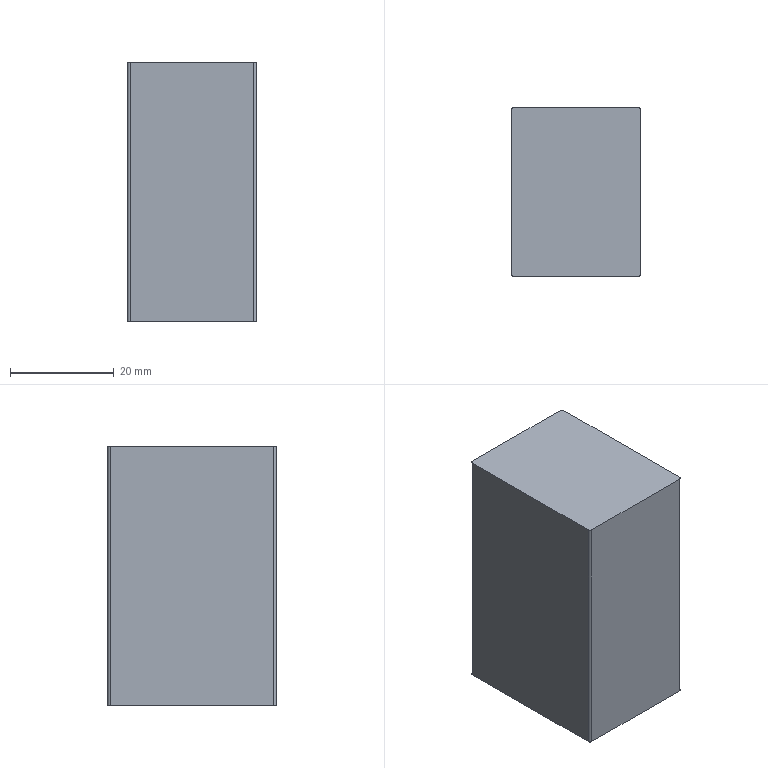Part | NX | features BREP 1 | 1 solid | 10 faces | box 24.892 x 32.505 x 50 mm | volume 40445 mm3 | plane 6 | cylinder 4 | commonest cylinder face diameters 1 x4
STEP:
#1=CARTESIAN_POINT('',(-11.946,16.253,-40.6));
#2=VERTEX_POINT('',#1);
#3=CARTESIAN_POINT('',(-12.446,15.753,-40.6));
#4=VERTEX_POINT('',#3);
#5=CARTESIAN_POINT('',(-11.946,15.753,-40.6));
#6=DIRECTION('',(0.,0.,1.));
#7=DIRECTION('',(1.,0.,0.));
#8=AXIS2_PLACEMENT_3D('',#5,#6,#7);
#9=CIRCLE('',#8,0.5);
#10=EDGE_CURVE('',#2,#4,#9,.T.);
#11=ORIENTED_EDGE('',*,*,#10,.F.);
#12=CARTESIAN_POINT('',(-11.946,16.253,-90.6));
#13=VERTEX_POINT('',#12);
#14=CARTESIAN_POINT('',(-11.946,16.253,-90.6));
#15=DIRECTION('',(0.,0.,1.));
#16=VECTOR('',#15,1000.);
#17=LINE('',#14,#16);
#18=EDGE_CURVE('',#13,#2,#17,.T.);
#19=ORIENTED_EDGE('',*,*,#18,.F.);
#20=CARTESIAN_POINT('',(-12.446,15.753,-90.6));
#21=VERTEX_POINT('',#20);
#22=CARTESIAN_POINT('',(-11.946,15.753,-90.6));
#23=DIRECTION('',(0.,0.,1.));
#24=DIRECTION('',(1.,0.,0.));
#25=AXIS2_PLACEMENT_3D('',#22,#23,#24);
#26=CIRCLE('',#25,0.5);
#27=EDGE_CURVE('',#13,#21,#26,.T.);
#28=ORIENTED_EDGE('',*,*,#27,.T.);
#29=CARTESIAN_POINT('',(-12.446,15.753,-90.6));
#30=DIRECTION('',(0.,0.,1.));
#31=VECTOR('',#30,1000.);
#32=LINE('',#29,#31);
#33=EDGE_CURVE('',#21,#4,#32,.T.);
#34=ORIENTED_EDGE('',*,*,#33,.T.);
#35=EDGE_LOOP('',(#11,#19,#28,#34));
#36=FACE_BOUND('',#35,.T.);
#37=CARTESIAN_POINT('',(-11.946,15.753,-90.6));
#38=DIRECTION('',(0.,0.,1.));
#39=DIRECTION('',(-1.,0.,0.));
#40=AXIS2_PLACEMENT_3D('',#37,#38,#39);
#41=CYLINDRICAL_SURFACE('',#40,0.5);
#42=ADVANCED_FACE('',(#36),#41,.T.);
#43=CARTESIAN_POINT('',(-12.446,-15.753,-40.6));
#44=VERTEX_POINT('',#43);
#45=CARTESIAN_POINT('',(-12.446,-15.753,-40.6));
#46=DIRECTION('',(0.,1.,0.));
#47=VECTOR('',#46,1000.);
#48=LINE('',#45,#47);
#49=EDGE_CURVE('',#44,#4,#48,.T.);
#50=ORIENTED_EDGE('',*,*,#49,.T.);
#51=ORIENTED_EDGE('',*,*,#33,.F.);
#52=CARTESIAN_POINT('',(-12.446,-15.753,-90.6));
#53=VERTEX_POINT('',#52);
#54=CARTESIAN_POINT('',(-12.446,-15.753,-90.6));
#55=DIRECTION('',(0.,1.,0.));
#56=VECTOR('',#55,1000.);
#57=LINE('',#54,#56);
#58=EDGE_CURVE('',#53,#21,#57,.T.);
#59=ORIENTED_EDGE('',*,*,#58,.F.);
#60=CARTESIAN_POINT('',(-12.446,-15.753,-90.6));
#61=DIRECTION('',(0.,0.,1.));
#62=VECTOR('',#61,1000.);
#63=LINE('',#60,#62);
#64=EDGE_CURVE('',#53,#44,#63,.T.);
#65=ORIENTED_EDGE('',*,*,#64,.T.);
#66=EDGE_LOOP('',(#50,#51,#59,#65));
#67=FACE_BOUND('',#66,.T.);
#68=CARTESIAN_POINT('',(-12.446,-15.753,-90.6));
#69=DIRECTION('',(1.,0.,0.));
#70=DIRECTION('',(0.,0.,1.));
#71=AXIS2_PLACEMENT_3D('',#68,#69,#70);
#72=PLANE('',#71);
#73=ADVANCED_FACE('',(#67),#72,.F.);
#74=CARTESIAN_POINT('',(-11.946,-16.253,-40.6));
#75=VERTEX_POINT('',#74);
#76=CARTESIAN_POINT('',(-11.946,-15.753,-40.6));
#77=DIRECTION('',(0.,0.,1.));
#78=DIRECTION('',(1.,0.,0.));
#79=AXIS2_PLACEMENT_3D('',#76,#77,#78);
#80=CIRCLE('',#79,0.5);
#81=EDGE_CURVE('',#44,#75,#80,.T.);
#82=ORIENTED_EDGE('',*,*,#81,.F.);
#83=ORIENTED_EDGE('',*,*,#64,.F.);
#84=CARTESIAN_POINT('',(-11.946,-16.253,-90.6));
#85=VERTEX_POINT('',#84);
#86=CARTESIAN_POINT('',(-11.946,-15.753,-90.6));
#87=DIRECTION('',(0.,0.,1.));
#88=DIRECTION('',(1.,0.,0.));
#89=AXIS2_PLACEMENT_3D('',#86,#87,#88);
#90=CIRCLE('',#89,0.5);
#91=EDGE_CURVE('',#53,#85,#90,.T.);
#92=ORIENTED_EDGE('',*,*,#91,.T.);
#93=CARTESIAN_POINT('',(-11.946,-16.253,-90.6));
#94=DIRECTION('',(0.,0.,1.));
#95=VECTOR('',#94,1000.);
#96=LINE('',#93,#95);
#97=EDGE_CURVE('',#85,#75,#96,.T.);
#98=ORIENTED_EDGE('',*,*,#97,.T.);
#99=EDGE_LOOP('',(#82,#83,#92,#98));
#100=FACE_BOUND('',#99,.T.);
#101=CARTESIAN_POINT('',(-11.946,-15.753,-90.6));
#102=DIRECTION('',(0.,0.,1.));
#103=DIRECTION('',(-1.,0.,0.));
#104=AXIS2_PLACEMENT_3D('',#101,#102,#103);
#105=CYLINDRICAL_SURFACE('',#104,0.5);
#106=ADVANCED_FACE('',(#100),#105,.T.);
#107=CARTESIAN_POINT('',(11.946,-16.253,-40.6));
#108=VERTEX_POINT('',#107);
#109=CARTESIAN_POINT('',(11.946,-16.253,-40.6));
#110=DIRECTION('',(-1.,0.,0.));
#111=VECTOR('',#110,1000.);
#112=LINE('',#109,#111);
#113=EDGE_CURVE('',#108,#75,#112,.T.);
#114=ORIENTED_EDGE('',*,*,#113,.T.);
#115=ORIENTED_EDGE('',*,*,#97,.F.);
#116=CARTESIAN_POINT('',(11.946,-16.253,-90.6));
#117=VERTEX_POINT('',#116);
#118=CARTESIAN_POINT('',(11.946,-16.253,-90.6));
#119=DIRECTION('',(-1.,0.,0.));
#120=VECTOR('',#119,1000.);
#121=LINE('',#118,#120);
#122=EDGE_CURVE('',#117,#85,#121,.T.);
#123=ORIENTED_EDGE('',*,*,#122,.F.);
#124=CARTESIAN_POINT('',(11.946,-16.253,-90.6));
#125=DIRECTION('',(0.,0.,1.));
#126=VECTOR('',#125,1000.);
#127=LINE('',#124,#126);
#128=EDGE_CURVE('',#117,#108,#127,.T.);
#129=ORIENTED_EDGE('',*,*,#128,.T.);
#130=EDGE_LOOP('',(#114,#115,#123,#129));
#131=FACE_BOUND('',#130,.T.);
#132=CARTESIAN_POINT('',(11.946,-16.253,-90.6));
#133=DIRECTION('',(0.,1.,0.));
#134=DIRECTION('',(0.,0.,-1.));
#135=AXIS2_PLACEMENT_3D('',#132,#133,#134);
#136=PLANE('',#135);
#137=ADVANCED_FACE('',(#131),#136,.F.);
#138=CARTESIAN_POINT('',(12.446,-15.753,-40.6));
#139=VERTEX_POINT('',#138);
#140=CARTESIAN_POINT('',(11.946,-15.753,-40.6));
#141=DIRECTION('',(0.,0.,1.));
#142=DIRECTION('',(1.,0.,0.));
#143=AXIS2_PLACEMENT_3D('',#140,#141,#142);
#144=CIRCLE('',#143,0.5);
#145=EDGE_CURVE('',#108,#139,#144,.T.);
#146=ORIENTED_EDGE('',*,*,#145,.F.);
#147=ORIENTED_EDGE('',*,*,#128,.F.);
#148=CARTESIAN_POINT('',(12.446,-15.753,-90.6));
#149=VERTEX_POINT('',#148);
#150=CARTESIAN_POINT('',(11.946,-15.753,-90.6));
#151=DIRECTION('',(0.,0.,1.));
#152=DIRECTION('',(1.,0.,0.));
#153=AXIS2_PLACEMENT_3D('',#150,#151,#152);
#154=CIRCLE('',#153,0.5);
#155=EDGE_CURVE('',#117,#149,#154,.T.);
#156=ORIENTED_EDGE('',*,*,#155,.T.);
#157=CARTESIAN_POINT('',(12.446,-15.753,-90.6));
#158=DIRECTION('',(0.,0.,1.));
#159=VECTOR('',#158,1000.);
#160=LINE('',#157,#159);
#161=EDGE_CURVE('',#149,#139,#160,.T.);
#162=ORIENTED_EDGE('',*,*,#161,.T.);
#163=EDGE_LOOP('',(#146,#147,#156,#162));
#164=FACE_BOUND('',#163,.T.);
#165=CARTESIAN_POINT('',(11.946,-15.753,-90.6));
#166=DIRECTION('',(0.,0.,1.));
#167=DIRECTION('',(-1.,0.,0.));
#168=AXIS2_PLACEMENT_3D('',#165,#166,#167);
#169=CYLINDRICAL_SURFACE('',#168,0.5);
#170=ADVANCED_FACE('',(#164),#169,.T.);
#171=CARTESIAN_POINT('',(12.446,15.753,-40.6));
#172=VERTEX_POINT('',#171);
#173=CARTESIAN_POINT('',(12.446,15.753,-40.6));
#174=DIRECTION('',(0.,-1.,0.));
#175=VECTOR('',#174,1000.);
#176=LINE('',#173,#175);
#177=EDGE_CURVE('',#172,#139,#176,.T.);
#178=ORIENTED_EDGE('',*,*,#177,.T.);
#179=ORIENTED_EDGE('',*,*,#161,.F.);
#180=CARTESIAN_POINT('',(12.446,15.753,-90.6));
#181=VERTEX_POINT('',#180);
#182=CARTESIAN_POINT('',(12.446,15.753,-90.6));
#183=DIRECTION('',(0.,-1.,0.));
#184=VECTOR('',#183,1000.);
#185=LINE('',#182,#184);
#186=EDGE_CURVE('',#181,#149,#185,.T.);
#187=ORIENTED_EDGE('',*,*,#186,.F.);
#188=CARTESIAN_POINT('',(12.446,15.753,-90.6));
#189=DIRECTION('',(0.,0.,1.));
#190=VECTOR('',#189,1000.);
#191=LINE('',#188,#190);
#192=EDGE_CURVE('',#181,#172,#191,.T.);
#193=ORIENTED_EDGE('',*,*,#192,.T.);
#194=EDGE_LOOP('',(#178,#179,#187,#193));
#195=FACE_BOUND('',#194,.T.);
#196=CARTESIAN_POINT('',(12.446,15.753,-90.6));
#197=DIRECTION('',(-1.,0.,0.));
#198=DIRECTION('',(0.,1.,0.));
#199=AXIS2_PLACEMENT_3D('',#196,#197,#198);
#200=PLANE('',#199);
#201=ADVANCED_FACE('',(#195),#200,.F.);
#202=CARTESIAN_POINT('',(11.946,16.253,-40.6));
#203=VERTEX_POINT('',#202);
#204=CARTESIAN_POINT('',(11.946,15.753,-40.6));
#205=DIRECTION('',(0.,0.,1.));
#206=DIRECTION('',(1.,0.,0.));
#207=AXIS2_PLACEMENT_3D('',#204,#205,#206);
#208=CIRCLE('',#207,0.5);
#209=EDGE_CURVE('',#172,#203,#208,.T.);
#210=ORIENTED_EDGE('',*,*,#209,.F.);
#211=ORIENTED_EDGE('',*,*,#192,.F.);
#212=CARTESIAN_POINT('',(11.946,16.253,-90.6));
#213=VERTEX_POINT('',#212);
#214=CARTESIAN_POINT('',(11.946,15.753,-90.6));
#215=DIRECTION('',(0.,0.,1.));
#216=DIRECTION('',(1.,0.,0.));
#217=AXIS2_PLACEMENT_3D('',#214,#215,#216);
#218=CIRCLE('',#217,0.5);
#219=EDGE_CURVE('',#181,#213,#218,.T.);
#220=ORIENTED_EDGE('',*,*,#219,.T.);
#221=CARTESIAN_POINT('',(11.946,16.253,-90.6));
#222=DIRECTION('',(0.,0.,1.));
#223=VECTOR('',#222,1000.);
#224=LINE('',#221,#223);
#225=EDGE_CURVE('',#213,#203,#224,.T.);
#226=ORIENTED_EDGE('',*,*,#225,.T.);
#227=EDGE_LOOP('',(#210,#211,#220,#226));
#228=FACE_BOUND('',#227,.T.);
#229=CARTESIAN_POINT('',(11.946,15.753,-90.6));
#230=DIRECTION('',(0.,0.,1.));
#231=DIRECTION('',(-1.,0.,0.));
#232=AXIS2_PLACEMENT_3D('',#229,#230,#231);
#233=CYLINDRICAL_SURFACE('',#232,0.5);
#234=ADVANCED_FACE('',(#228),#233,.T.);
#235=CARTESIAN_POINT('',(-11.946,16.253,-40.6));
#236=DIRECTION('',(1.,0.,0.));
#237=VECTOR('',#236,1000.);
#238=LINE('',#235,#237);
#239=EDGE_CURVE('',#2,#203,#238,.T.);
#240=ORIENTED_EDGE('',*,*,#239,.T.);
#241=ORIENTED_EDGE('',*,*,#225,.F.);
#242=CARTESIAN_POINT('',(-11.946,16.253,-90.6));
#243=DIRECTION('',(1.,0.,0.));
#244=VECTOR('',#243,1000.);
#245=LINE('',#242,#244);
#246=EDGE_CURVE('',#13,#213,#245,.T.);
#247=ORIENTED_EDGE('',*,*,#246,.F.);
#248=ORIENTED_EDGE('',*,*,#18,.T.);
#249=EDGE_LOOP('',(#240,#241,#247,#248));
#250=FACE_BOUND('',#249,.T.);
#251=CARTESIAN_POINT('',(-11.946,16.253,-90.6));
#252=DIRECTION('',(0.,-1.,0.));
#253=DIRECTION('',(0.,0.,1.));
#254=AXIS2_PLACEMENT_3D('',#251,#252,#253);
#255=PLANE('',#254);
#256=ADVANCED_FACE('',(#250),#255,.F.);
#257=ORIENTED_EDGE('',*,*,#27,.F.);
#258=ORIENTED_EDGE('',*,*,#246,.T.);
#259=ORIENTED_EDGE('',*,*,#219,.F.);
#260=ORIENTED_EDGE('',*,*,#186,.T.);
#261=ORIENTED_EDGE('',*,*,#155,.F.);
#262=ORIENTED_EDGE('',*,*,#122,.T.);
#263=ORIENTED_EDGE('',*,*,#91,.F.);
#264=ORIENTED_EDGE('',*,*,#58,.T.);
#265=EDGE_LOOP('',(#257,#258,#259,#260,#261,#262,#263,#264));
#266=FACE_BOUND('',#265,.T.);
#267=CARTESIAN_POINT('',(-11.946,15.753,-90.6));
#268=DIRECTION('',(0.,0.,1.));
#269=DIRECTION('',(-1.,0.,0.));
#270=AXIS2_PLACEMENT_3D('',#267,#268,#269);
#271=PLANE('',#270);
#272=ADVANCED_FACE('',(#266),#271,.F.);
#273=ORIENTED_EDGE('',*,*,#10,.T.);
#274=ORIENTED_EDGE('',*,*,#49,.F.);
#275=ORIENTED_EDGE('',*,*,#81,.T.);
#276=ORIENTED_EDGE('',*,*,#113,.F.);
#277=ORIENTED_EDGE('',*,*,#145,.T.);
#278=ORIENTED_EDGE('',*,*,#177,.F.);
#279=ORIENTED_EDGE('',*,*,#209,.T.);
#280=ORIENTED_EDGE('',*,*,#239,.F.);
#281=EDGE_LOOP('',(#273,#274,#275,#276,#277,#278,#279,#280));
#282=FACE_BOUND('',#281,.T.);
#283=CARTESIAN_POINT('',(-11.946,15.753,-40.6));
#284=DIRECTION('',(0.,0.,1.));
#285=DIRECTION('',(-1.,0.,0.));
#286=AXIS2_PLACEMENT_3D('',#283,#284,#285);
#287=PLANE('',#286);
#288=ADVANCED_FACE('',(#282),#287,.T.);
#289=CLOSED_SHELL('',(#42,#73,#106,#137,#170,#201,#234,#256,#272,#288));
#290=MANIFOLD_SOLID_BREP('',#289);
#291=(LENGTH_UNIT()NAMED_UNIT(*)SI_UNIT(.MILLI.,.METRE.));
#292=UNCERTAINTY_MEASURE_WITH_UNIT(LENGTH_MEASURE(0.00001),#291,'','');
#293=(NAMED_UNIT(*)PLANE_ANGLE_UNIT()SI_UNIT($,.RADIAN.));
#294=(NAMED_UNIT(*)SI_UNIT($,.STERADIAN.)SOLID_ANGLE_UNIT());
#295=(GEOMETRIC_REPRESENTATION_CONTEXT(3)GLOBAL_UNCERTAINTY_ASSIGNED_CONTEXT((#292))GLOBAL_UNIT_ASSIGNED_CONTEXT((#291,#293,#294))REPRESENTATION_CONTEXT('',''));
#296=ADVANCED_BREP_SHAPE_REPRESENTATION('',(#290),#295);